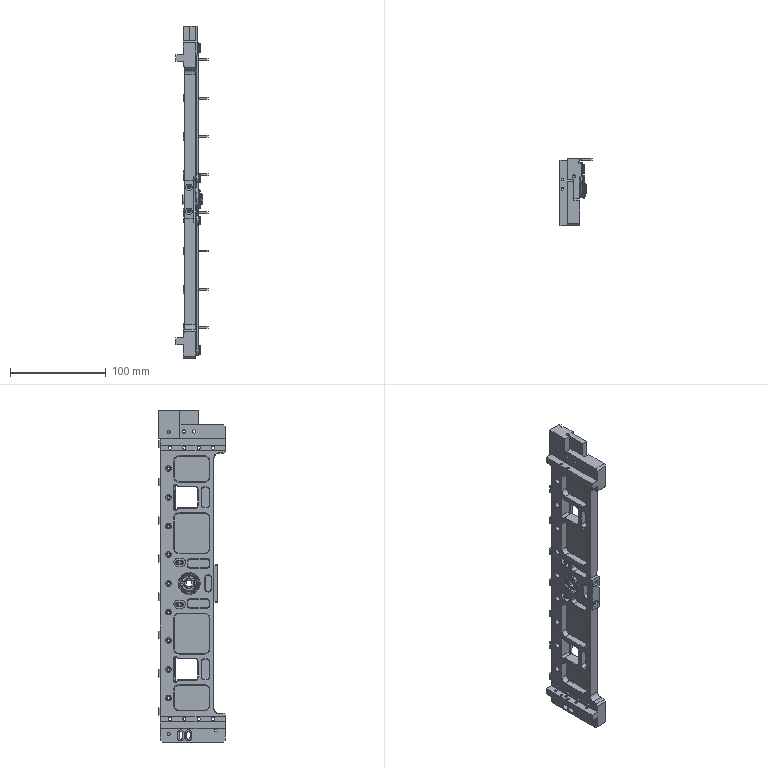Part | NX | features BREP 15 | 37 solids | 1550 faces | box 33.5 x 70 x 347.5 mm | volume 189578 mm3 | cylinder 666 | plane 644 | cone 104 | sphere 56 | spline 48 | torus 32 | commonest cylinder face diameters 0.46 x120 4 x88 3.4 x60 6 x46 10 x45 2.5 x44